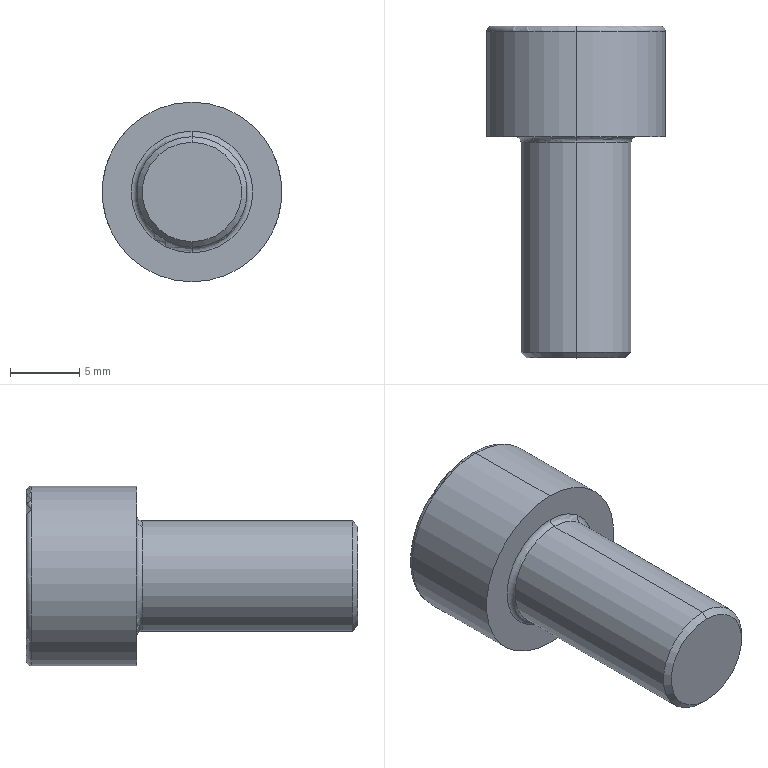Part | STEP file | 1 solid | 20 faces | box 13 x 24 x 13 mm | volume 1739 mm3 | plane 10 | torus 4 | cylinder 4 | cone 2 | commonest cylinder face diameters 8 x2 13 x2
STEP:
#1=CARTESIAN_POINT('',(0.,-16.,-3.6));
#2=VERTEX_POINT('',#1);
#3=CARTESIAN_POINT('',(0.,-16.,3.6));
#4=VERTEX_POINT('',#3);
#5=CARTESIAN_POINT('',(0.,-16.,0.));
#6=DIRECTION('',(0.,-1.,0.));
#7=DIRECTION('',(0.,0.,-1.));
#8=AXIS2_PLACEMENT_3D('',#5,#6,#7);
#9=CIRCLE('',#8,3.6);
#10=EDGE_CURVE('',#2,#4,#9,.T.);
#11=ORIENTED_EDGE('',*,*,#10,.F.);
#12=CARTESIAN_POINT('',(0.,-15.6,-4.));
#13=VERTEX_POINT('',#12);
#14=CARTESIAN_POINT('',(0.,-16.,-3.6));
#15=DIRECTION('',(0.,0.7071,-0.7071));
#16=VECTOR('',#15,1000.);
#17=LINE('',#14,#16);
#18=EDGE_CURVE('',#2,#13,#17,.T.);
#19=ORIENTED_EDGE('',*,*,#18,.T.);
#20=CARTESIAN_POINT('',(0.,-15.6,4.));
#21=VERTEX_POINT('',#20);
#22=CARTESIAN_POINT('',(0.,-15.6,0.));
#23=DIRECTION('',(0.,1.,0.));
#24=DIRECTION('',(0.,0.,-1.));
#25=AXIS2_PLACEMENT_3D('',#22,#23,#24);
#26=CIRCLE('',#25,4.);
#27=EDGE_CURVE('',#21,#13,#26,.T.);
#28=ORIENTED_EDGE('',*,*,#27,.F.);
#29=CARTESIAN_POINT('',(0.,-16.,3.6));
#30=DIRECTION('',(0.,0.7071,0.7071));
#31=VECTOR('',#30,1000.);
#32=LINE('',#29,#31);
#33=EDGE_CURVE('',#4,#21,#32,.T.);
#34=ORIENTED_EDGE('',*,*,#33,.F.);
#35=EDGE_LOOP('',(#11,#19,#28,#34));
#36=FACE_OUTER_BOUND('',#35,.T.);
#37=CARTESIAN_POINT('',(0.,-16.,0.));
#38=DIRECTION('',(0.,1.,0.));
#39=DIRECTION('',(0.,0.,1.));
#40=AXIS2_PLACEMENT_3D('',#37,#38,#39);
#41=CONICAL_SURFACE('',#40,3.6,0.7854);
#42=ADVANCED_FACE('',(#36),#41,.T.);
#43=CARTESIAN_POINT('',(0.,7.6,-6.5));
#44=VERTEX_POINT('',#43);
#45=CARTESIAN_POINT('',(0.,7.6,6.5));
#46=VERTEX_POINT('',#45);
#47=CARTESIAN_POINT('',(0.,7.6,0.));
#48=DIRECTION('',(0.,-1.,0.));
#49=DIRECTION('',(0.,0.,1.));
#50=AXIS2_PLACEMENT_3D('',#47,#48,#49);
#51=CIRCLE('',#50,6.5);
#52=EDGE_CURVE('',#44,#46,#51,.T.);
#53=ORIENTED_EDGE('',*,*,#52,.F.);
#54=CARTESIAN_POINT('',(0.,8.,-6.1));
#55=VERTEX_POINT('',#54);
#56=CARTESIAN_POINT('',(0.,7.6,-6.1));
#57=DIRECTION('',(1.,0.,0.));
#58=DIRECTION('',(0.,0.,-1.));
#59=AXIS2_PLACEMENT_3D('',#56,#57,#58);
#60=CIRCLE('',#59,0.4);
#61=EDGE_CURVE('',#44,#55,#60,.T.);
#62=ORIENTED_EDGE('',*,*,#61,.T.);
#63=CARTESIAN_POINT('',(0.,8.,6.1));
#64=VERTEX_POINT('',#63);
#65=CARTESIAN_POINT('',(0.,8.,0.));
#66=DIRECTION('',(0.,1.,0.));
#67=DIRECTION('',(0.,0.,1.));
#68=AXIS2_PLACEMENT_3D('',#65,#66,#67);
#69=CIRCLE('',#68,6.1);
#70=EDGE_CURVE('',#64,#55,#69,.T.);
#71=ORIENTED_EDGE('',*,*,#70,.F.);
#72=CARTESIAN_POINT('',(0.,7.6,6.1));
#73=DIRECTION('',(-1.,0.,0.));
#74=DIRECTION('',(0.,0.,1.));
#75=AXIS2_PLACEMENT_3D('',#72,#73,#74);
#76=CIRCLE('',#75,0.4);
#77=EDGE_CURVE('',#46,#64,#76,.T.);
#78=ORIENTED_EDGE('',*,*,#77,.F.);
#79=EDGE_LOOP('',(#53,#62,#71,#78));
#80=FACE_OUTER_BOUND('',#79,.T.);
#81=CARTESIAN_POINT('',(0.,7.6,0.));
#82=DIRECTION('',(0.,1.,0.));
#83=DIRECTION('',(0.,0.,1.));
#84=AXIS2_PLACEMENT_3D('',#81,#82,#83);
#85=TOROIDAL_SURFACE('',#84,6.1,0.4);
#86=ADVANCED_FACE('',(#80),#85,.T.);
#87=CARTESIAN_POINT('',(0.,-0.4,4.));
#88=VERTEX_POINT('',#87);
#89=CARTESIAN_POINT('',(0.,-0.4,-4.));
#90=VERTEX_POINT('',#89);
#91=CARTESIAN_POINT('',(0.,-0.4,0.));
#92=DIRECTION('',(0.,-1.,0.));
#93=DIRECTION('',(0.,0.,-1.));
#94=AXIS2_PLACEMENT_3D('',#91,#92,#93);
#95=CIRCLE('',#94,4.);
#96=EDGE_CURVE('',#88,#90,#95,.T.);
#97=ORIENTED_EDGE('',*,*,#96,.F.);
#98=CARTESIAN_POINT('',(0.,0.,4.4));
#99=VERTEX_POINT('',#98);
#100=CARTESIAN_POINT('',(0.,-0.4,4.4));
#101=DIRECTION('',(1.,0.,0.));
#102=DIRECTION('',(0.,0.,-1.));
#103=AXIS2_PLACEMENT_3D('',#100,#101,#102);
#104=CIRCLE('',#103,0.4);
#105=EDGE_CURVE('',#88,#99,#104,.T.);
#106=ORIENTED_EDGE('',*,*,#105,.T.);
#107=CARTESIAN_POINT('',(0.,0.,-4.4));
#108=VERTEX_POINT('',#107);
#109=CARTESIAN_POINT('',(0.,0.,0.));
#110=DIRECTION('',(0.,1.,0.));
#111=DIRECTION('',(0.,0.,-1.));
#112=AXIS2_PLACEMENT_3D('',#109,#110,#111);
#113=CIRCLE('',#112,4.4);
#114=EDGE_CURVE('',#108,#99,#113,.T.);
#115=ORIENTED_EDGE('',*,*,#114,.F.);
#116=CARTESIAN_POINT('',(0.,-0.4,-4.4));
#117=DIRECTION('',(-1.,0.,0.));
#118=DIRECTION('',(0.,0.,1.));
#119=AXIS2_PLACEMENT_3D('',#116,#117,#118);
#120=CIRCLE('',#119,0.4);
#121=EDGE_CURVE('',#90,#108,#120,.T.);
#122=ORIENTED_EDGE('',*,*,#121,.F.);
#123=EDGE_LOOP('',(#97,#106,#115,#122));
#124=FACE_OUTER_BOUND('',#123,.T.);
#125=CARTESIAN_POINT('',(0.,-0.4,0.));
#126=DIRECTION('',(0.,-1.,0.));
#127=DIRECTION('',(0.,0.,-1.));
#128=AXIS2_PLACEMENT_3D('',#125,#126,#127);
#129=TOROIDAL_SURFACE('',#128,4.4,0.4);
#130=ADVANCED_FACE('',(#124),#129,.F.);
#131=CARTESIAN_POINT('',(0.,-0.4,0.));
#132=DIRECTION('',(0.,-1.,0.));
#133=DIRECTION('',(0.,0.,-1.));
#134=AXIS2_PLACEMENT_3D('',#131,#132,#133);
#135=CIRCLE('',#134,4.);
#136=EDGE_CURVE('',#90,#88,#135,.T.);
#137=ORIENTED_EDGE('',*,*,#136,.T.);
#138=CARTESIAN_POINT('',(0.,0.,4.));
#139=DIRECTION('',(0.,-1.,0.));
#140=VECTOR('',#139,1000.);
#141=LINE('',#138,#140);
#142=EDGE_CURVE('',#88,#21,#141,.T.);
#143=ORIENTED_EDGE('',*,*,#142,.T.);
#144=ORIENTED_EDGE('',*,*,#27,.T.);
#145=CARTESIAN_POINT('',(0.,0.,-4.));
#146=DIRECTION('',(0.,-1.,0.));
#147=VECTOR('',#146,1000.);
#148=LINE('',#145,#147);
#149=EDGE_CURVE('',#90,#13,#148,.T.);
#150=ORIENTED_EDGE('',*,*,#149,.F.);
#151=EDGE_LOOP('',(#137,#143,#144,#150));
#152=FACE_OUTER_BOUND('',#151,.T.);
#153=CARTESIAN_POINT('',(0.,0.,0.));
#154=DIRECTION('',(0.,-1.,0.));
#155=DIRECTION('',(0.,0.,-1.));
#156=AXIS2_PLACEMENT_3D('',#153,#154,#155);
#157=CYLINDRICAL_SURFACE('',#156,4.);
#158=ADVANCED_FACE('',(#152),#157,.T.);
#159=ORIENTED_EDGE('',*,*,#52,.T.);
#160=CARTESIAN_POINT('',(0.,0.,6.5));
#161=VERTEX_POINT('',#160);
#162=CARTESIAN_POINT('',(0.,0.,6.5));
#163=DIRECTION('',(0.,-1.,0.));
#164=VECTOR('',#163,1000.);
#165=LINE('',#162,#164);
#166=EDGE_CURVE('',#46,#161,#165,.T.);
#167=ORIENTED_EDGE('',*,*,#166,.T.);
#168=CARTESIAN_POINT('',(0.,0.,-6.5));
#169=VERTEX_POINT('',#168);
#170=CARTESIAN_POINT('',(0.,0.,0.));
#171=DIRECTION('',(0.,-1.,0.));
#172=DIRECTION('',(0.,0.,-1.));
#173=AXIS2_PLACEMENT_3D('',#170,#171,#172);
#174=CIRCLE('',#173,6.5);
#175=EDGE_CURVE('',#169,#161,#174,.T.);
#176=ORIENTED_EDGE('',*,*,#175,.F.);
#177=CARTESIAN_POINT('',(0.,0.,-6.5));
#178=DIRECTION('',(0.,-1.,0.));
#179=VECTOR('',#178,1000.);
#180=LINE('',#177,#179);
#181=EDGE_CURVE('',#44,#169,#180,.T.);
#182=ORIENTED_EDGE('',*,*,#181,.F.);
#183=EDGE_LOOP('',(#159,#167,#176,#182));
#184=FACE_OUTER_BOUND('',#183,.T.);
#185=CARTESIAN_POINT('',(0.,0.,0.));
#186=DIRECTION('',(0.,-1.,0.));
#187=DIRECTION('',(0.,0.,-1.));
#188=AXIS2_PLACEMENT_3D('',#185,#186,#187);
#189=CYLINDRICAL_SURFACE('',#188,6.5);
#190=ADVANCED_FACE('',(#184),#189,.T.);
#191=ORIENTED_EDGE('',*,*,#70,.T.);
#192=CARTESIAN_POINT('',(0.,8.,0.));
#193=DIRECTION('',(0.,1.,0.));
#194=DIRECTION('',(0.,0.,1.));
#195=AXIS2_PLACEMENT_3D('',#192,#193,#194);
#196=CIRCLE('',#195,6.1);
#197=EDGE_CURVE('',#55,#64,#196,.T.);
#198=ORIENTED_EDGE('',*,*,#197,.T.);
#199=EDGE_LOOP('',(#191,#198));
#200=FACE_OUTER_BOUND('',#199,.T.);
#201=CARTESIAN_POINT('',(0.,8.,-3.464));
#202=VERTEX_POINT('',#201);
#203=CARTESIAN_POINT('',(-3.,8.,-1.732));
#204=VERTEX_POINT('',#203);
#205=CARTESIAN_POINT('',(0.,8.,-3.464));
#206=DIRECTION('',(-0.866,0.,0.5));
#207=VECTOR('',#206,1000.);
#208=LINE('',#205,#207);
#209=EDGE_CURVE('',#202,#204,#208,.T.);
#210=ORIENTED_EDGE('',*,*,#209,.F.);
#211=CARTESIAN_POINT('',(3.,8.,-1.732));
#212=VERTEX_POINT('',#211);
#213=CARTESIAN_POINT('',(3.,8.,-1.732));
#214=DIRECTION('',(-0.866,0.,-0.5));
#215=VECTOR('',#214,1000.);
#216=LINE('',#213,#215);
#217=EDGE_CURVE('',#212,#202,#216,.T.);
#218=ORIENTED_EDGE('',*,*,#217,.F.);
#219=CARTESIAN_POINT('',(3.,8.,1.732));
#220=VERTEX_POINT('',#219);
#221=CARTESIAN_POINT('',(3.,8.,1.732));
#222=DIRECTION('',(0.,0.,-1.));
#223=VECTOR('',#222,1000.);
#224=LINE('',#221,#223);
#225=EDGE_CURVE('',#220,#212,#224,.T.);
#226=ORIENTED_EDGE('',*,*,#225,.F.);
#227=CARTESIAN_POINT('',(0.,8.,3.464));
#228=VERTEX_POINT('',#227);
#229=CARTESIAN_POINT('',(0.,8.,3.464));
#230=DIRECTION('',(0.866,0.,-0.5));
#231=VECTOR('',#230,1000.);
#232=LINE('',#229,#231);
#233=EDGE_CURVE('',#228,#220,#232,.T.);
#234=ORIENTED_EDGE('',*,*,#233,.F.);
#235=CARTESIAN_POINT('',(-3.,8.,1.732));
#236=VERTEX_POINT('',#235);
#237=CARTESIAN_POINT('',(-3.,8.,1.732));
#238=DIRECTION('',(0.866,0.,0.5));
#239=VECTOR('',#238,1000.);
#240=LINE('',#237,#239);
#241=EDGE_CURVE('',#236,#228,#240,.T.);
#242=ORIENTED_EDGE('',*,*,#241,.F.);
#243=CARTESIAN_POINT('',(-3.,8.,-1.732));
#244=DIRECTION('',(0.,0.,1.));
#245=VECTOR('',#244,1000.);
#246=LINE('',#243,#245);
#247=EDGE_CURVE('',#204,#236,#246,.T.);
#248=ORIENTED_EDGE('',*,*,#247,.F.);
#249=EDGE_LOOP('',(#210,#218,#226,#234,#242,#248));
#250=FACE_BOUND('',#249,.T.);
#251=CARTESIAN_POINT('',(0.,8.,0.));
#252=DIRECTION('',(0.,1.,0.));
#253=DIRECTION('',(0.,0.,1.));
#254=AXIS2_PLACEMENT_3D('',#251,#252,#253);
#255=PLANE('',#254);
#256=ADVANCED_FACE('',(#200,#250),#255,.T.);
#257=ORIENTED_EDGE('',*,*,#166,.F.);
#258=CARTESIAN_POINT('',(0.,7.6,0.));
#259=DIRECTION('',(0.,-1.,0.));
#260=DIRECTION('',(0.,0.,1.));
#261=AXIS2_PLACEMENT_3D('',#258,#259,#260);
#262=CIRCLE('',#261,6.5);
#263=EDGE_CURVE('',#46,#44,#262,.T.);
#264=ORIENTED_EDGE('',*,*,#263,.T.);
#265=ORIENTED_EDGE('',*,*,#181,.T.);
#266=CARTESIAN_POINT('',(0.,0.,0.));
#267=DIRECTION('',(0.,-1.,0.));
#268=DIRECTION('',(0.,0.,-1.));
#269=AXIS2_PLACEMENT_3D('',#266,#267,#268);
#270=CIRCLE('',#269,6.5);
#271=EDGE_CURVE('',#161,#169,#270,.T.);
#272=ORIENTED_EDGE('',*,*,#271,.F.);
#273=EDGE_LOOP('',(#257,#264,#265,#272));
#274=FACE_OUTER_BOUND('',#273,.T.);
#275=CARTESIAN_POINT('',(0.,0.,0.));
#276=DIRECTION('',(0.,-1.,0.));
#277=DIRECTION('',(0.,0.,-1.));
#278=AXIS2_PLACEMENT_3D('',#275,#276,#277);
#279=CYLINDRICAL_SURFACE('',#278,6.5);
#280=ADVANCED_FACE('',(#274),#279,.T.);
#281=ORIENTED_EDGE('',*,*,#114,.T.);
#282=CARTESIAN_POINT('',(0.,0.,0.));
#283=DIRECTION('',(0.,1.,0.));
#284=DIRECTION('',(0.,0.,-1.));
#285=AXIS2_PLACEMENT_3D('',#282,#283,#284);
#286=CIRCLE('',#285,4.4);
#287=EDGE_CURVE('',#99,#108,#286,.T.);
#288=ORIENTED_EDGE('',*,*,#287,.T.);
#289=EDGE_LOOP('',(#281,#288));
#290=FACE_BOUND('',#289,.T.);
#291=ORIENTED_EDGE('',*,*,#175,.T.);
#292=ORIENTED_EDGE('',*,*,#271,.T.);
#293=EDGE_LOOP('',(#291,#292));
#294=FACE_OUTER_BOUND('',#293,.T.);
#295=CARTESIAN_POINT('',(6.5,0.,0.));
#296=DIRECTION('',(0.,-1.,0.));
#297=DIRECTION('',(0.,0.,-1.));
#298=AXIS2_PLACEMENT_3D('',#295,#296,#297);
#299=PLANE('',#298);
#300=ADVANCED_FACE('',(#290,#294),#299,.T.);
#301=ORIENTED_EDGE('',*,*,#142,.F.);
#302=ORIENTED_EDGE('',*,*,#96,.T.);
#303=ORIENTED_EDGE('',*,*,#149,.T.);
#304=CARTESIAN_POINT('',(0.,-15.6,0.));
#305=DIRECTION('',(0.,1.,0.));
#306=DIRECTION('',(0.,0.,-1.));
#307=AXIS2_PLACEMENT_3D('',#304,#305,#306);
#308=CIRCLE('',#307,4.);
#309=EDGE_CURVE('',#13,#21,#308,.T.);
#310=ORIENTED_EDGE('',*,*,#309,.T.);
#311=EDGE_LOOP('',(#301,#302,#303,#310));
#312=FACE_OUTER_BOUND('',#311,.T.);
#313=CARTESIAN_POINT('',(0.,0.,0.));
#314=DIRECTION('',(0.,-1.,0.));
#315=DIRECTION('',(0.,0.,-1.));
#316=AXIS2_PLACEMENT_3D('',#313,#314,#315);
#317=CYLINDRICAL_SURFACE('',#316,4.);
#318=ADVANCED_FACE('',(#312),#317,.T.);
#319=CARTESIAN_POINT('',(0.,-16.,0.));
#320=DIRECTION('',(0.,-1.,0.));
#321=DIRECTION('',(0.,0.,-1.));
#322=AXIS2_PLACEMENT_3D('',#319,#320,#321);
#323=CIRCLE('',#322,3.6);
#324=EDGE_CURVE('',#4,#2,#323,.T.);
#325=ORIENTED_EDGE('',*,*,#324,.T.);
#326=ORIENTED_EDGE('',*,*,#10,.T.);
#327=EDGE_LOOP('',(#325,#326));
#328=FACE_OUTER_BOUND('',#327,.T.);
#329=CARTESIAN_POINT('',(4.,-16.,0.));
#330=DIRECTION('',(0.,-1.,0.));
#331=DIRECTION('',(0.,0.,-1.));
#332=AXIS2_PLACEMENT_3D('',#329,#330,#331);
#333=PLANE('',#332);
#334=ADVANCED_FACE('',(#328),#333,.T.);
#335=ORIENTED_EDGE('',*,*,#209,.T.);
#336=CARTESIAN_POINT('',(-3.,4.,-1.732));
#337=VERTEX_POINT('',#336);
#338=CARTESIAN_POINT('',(-3.,4.,-1.732));
#339=DIRECTION('',(0.,1.,0.));
#340=VECTOR('',#339,1000.);
#341=LINE('',#338,#340);
#342=EDGE_CURVE('',#337,#204,#341,.T.);
#343=ORIENTED_EDGE('',*,*,#342,.F.);
#344=CARTESIAN_POINT('',(0.,4.,-3.464));
#345=VERTEX_POINT('',#344);
#346=CARTESIAN_POINT('',(0.,4.,-3.464));
#347=DIRECTION('',(-0.866,0.,0.5));
#348=VECTOR('',#347,1000.);
#349=LINE('',#346,#348);
#350=EDGE_CURVE('',#345,#337,#349,.T.);
#351=ORIENTED_EDGE('',*,*,#350,.F.);
#352=CARTESIAN_POINT('',(0.,4.,-3.464));
#353=DIRECTION('',(0.,1.,0.));
#354=VECTOR('',#353,1000.);
#355=LINE('',#352,#354);
#356=EDGE_CURVE('',#345,#202,#355,.T.);
#357=ORIENTED_EDGE('',*,*,#356,.T.);
#358=EDGE_LOOP('',(#335,#343,#351,#357));
#359=FACE_OUTER_BOUND('',#358,.T.);
#360=CARTESIAN_POINT('',(0.,4.,-3.464));
#361=DIRECTION('',(-0.5,0.,-0.866));
#362=DIRECTION('',(-0.866,0.,0.5));
#363=AXIS2_PLACEMENT_3D('',#360,#361,#362);
#364=PLANE('',#363);
#365=ADVANCED_FACE('',(#359),#364,.F.);
#366=ORIENTED_EDGE('',*,*,#217,.T.);
#367=ORIENTED_EDGE('',*,*,#356,.F.);
#368=CARTESIAN_POINT('',(3.,4.,-1.732));
#369=VERTEX_POINT('',#368);
#370=CARTESIAN_POINT('',(3.,4.,-1.732));
#371=DIRECTION('',(-0.866,0.,-0.5));
#372=VECTOR('',#371,1000.);
#373=LINE('',#370,#372);
#374=EDGE_CURVE('',#369,#345,#373,.T.);
#375=ORIENTED_EDGE('',*,*,#374,.F.);
#376=CARTESIAN_POINT('',(3.,4.,-1.732));
#377=DIRECTION('',(0.,1.,0.));
#378=VECTOR('',#377,1000.);
#379=LINE('',#376,#378);
#380=EDGE_CURVE('',#369,#212,#379,.T.);
#381=ORIENTED_EDGE('',*,*,#380,.T.);
#382=EDGE_LOOP('',(#366,#367,#375,#381));
#383=FACE_OUTER_BOUND('',#382,.T.);
#384=CARTESIAN_POINT('',(3.,4.,-1.732));
#385=DIRECTION('',(0.5,0.,-0.866));
#386=DIRECTION('',(-0.866,0.,-0.5));
#387=AXIS2_PLACEMENT_3D('',#384,#385,#386);
#388=PLANE('',#387);
#389=ADVANCED_FACE('',(#383),#388,.F.);
#390=ORIENTED_EDGE('',*,*,#225,.T.);
#391=ORIENTED_EDGE('',*,*,#380,.F.);
#392=CARTESIAN_POINT('',(3.,4.,1.732));
#393=VERTEX_POINT('',#392);
#394=CARTESIAN_POINT('',(3.,4.,1.732));
#395=DIRECTION('',(0.,0.,-1.));
#396=VECTOR('',#395,1000.);
#397=LINE('',#394,#396);
#398=EDGE_CURVE('',#393,#369,#397,.T.);
#399=ORIENTED_EDGE('',*,*,#398,.F.);
#400=CARTESIAN_POINT('',(3.,4.,1.732));
#401=DIRECTION('',(0.,1.,0.));
#402=VECTOR('',#401,1000.);
#403=LINE('',#400,#402);
#404=EDGE_CURVE('',#393,#220,#403,.T.);
#405=ORIENTED_EDGE('',*,*,#404,.T.);
#406=EDGE_LOOP('',(#390,#391,#399,#405));
#407=FACE_OUTER_BOUND('',#406,.T.);
#408=CARTESIAN_POINT('',(3.,4.,1.732));
#409=DIRECTION('',(1.,0.,0.));
#410=DIRECTION('',(0.,0.,-1.));
#411=AXIS2_PLACEMENT_3D('',#408,#409,#410);
#412=PLANE('',#411);
#413=ADVANCED_FACE('',(#407),#412,.F.);
#414=ORIENTED_EDGE('',*,*,#233,.T.);
#415=ORIENTED_EDGE('',*,*,#404,.F.);
#416=CARTESIAN_POINT('',(0.,4.,3.464));
#417=VERTEX_POINT('',#416);
#418=CARTESIAN_POINT('',(0.,4.,3.464));
#419=DIRECTION('',(0.866,0.,-0.5));
#420=VECTOR('',#419,1000.);
#421=LINE('',#418,#420);
#422=EDGE_CURVE('',#417,#393,#421,.T.);
#423=ORIENTED_EDGE('',*,*,#422,.F.);
#424=CARTESIAN_POINT('',(0.,4.,3.464));
#425=DIRECTION('',(0.,1.,0.));
#426=VECTOR('',#425,1000.);
#427=LINE('',#424,#426);
#428=EDGE_CURVE('',#417,#228,#427,.T.);
#429=ORIENTED_EDGE('',*,*,#428,.T.);
#430=EDGE_LOOP('',(#414,#415,#423,#429));
#431=FACE_OUTER_BOUND('',#430,.T.);
#432=CARTESIAN_POINT('',(0.,4.,3.464));
#433=DIRECTION('',(0.5,0.,0.866));
#434=DIRECTION('',(0.866,0.,-0.5));
#435=AXIS2_PLACEMENT_3D('',#432,#433,#434);
#436=PLANE('',#435);
#437=ADVANCED_FACE('',(#431),#436,.F.);
#438=ORIENTED_EDGE('',*,*,#241,.T.);
#439=ORIENTED_EDGE('',*,*,#428,.F.);
#440=CARTESIAN_POINT('',(-3.,4.,1.732));
#441=VERTEX_POINT('',#440);
#442=CARTESIAN_POINT('',(-3.,4.,1.732));
#443=DIRECTION('',(0.866,0.,0.5));
#444=VECTOR('',#443,1000.);
#445=LINE('',#442,#444);
#446=EDGE_CURVE('',#441,#417,#445,.T.);
#447=ORIENTED_EDGE('',*,*,#446,.F.);
#448=CARTESIAN_POINT('',(-3.,4.,1.732));
#449=DIRECTION('',(0.,1.,0.));
#450=VECTOR('',#449,1000.);
#451=LINE('',#448,#450);
#452=EDGE_CURVE('',#441,#236,#451,.T.);
#453=ORIENTED_EDGE('',*,*,#452,.T.);
#454=EDGE_LOOP('',(#438,#439,#447,#453));
#455=FACE_OUTER_BOUND('',#454,.T.);
#456=CARTESIAN_POINT('',(-3.,4.,1.732));
#457=DIRECTION('',(-0.5,0.,0.866));
#458=DIRECTION('',(0.866,0.,0.5));
#459=AXIS2_PLACEMENT_3D('',#456,#457,#458);
#460=PLANE('',#459);
#461=ADVANCED_FACE('',(#455),#460,.F.);
#462=ORIENTED_EDGE('',*,*,#247,.T.);
#463=ORIENTED_EDGE('',*,*,#452,.F.);
#464=CARTESIAN_POINT('',(-3.,4.,-1.732));
#465=DIRECTION('',(0.,0.,1.));
#466=VECTOR('',#465,1000.);
#467=LINE('',#464,#466);
#468=EDGE_CURVE('',#337,#441,#467,.T.);
#469=ORIENTED_EDGE('',*,*,#468,.F.);
#470=ORIENTED_EDGE('',*,*,#342,.T.);
#471=EDGE_LOOP('',(#462,#463,#469,#470));
#472=FACE_OUTER_BOUND('',#471,.T.);
#473=CARTESIAN_POINT('',(-3.,4.,-1.732));
#474=DIRECTION('',(-1.,0.,0.));
#475=DIRECTION('',(0.,0.,1.));
#476=AXIS2_PLACEMENT_3D('',#473,#474,#475);
#477=PLANE('',#476);
#478=ADVANCED_FACE('',(#472),#477,.F.);
#479=ORIENTED_EDGE('',*,*,#350,.T.);
#480=ORIENTED_EDGE('',*,*,#468,.T.);
#481=ORIENTED_EDGE('',*,*,#446,.T.);
#482=ORIENTED_EDGE('',*,*,#422,.T.);
#483=ORIENTED_EDGE('',*,*,#398,.T.);
#484=ORIENTED_EDGE('',*,*,#374,.T.);
#485=EDGE_LOOP('',(#479,#480,#481,#482,#483,#484));
#486=FACE_OUTER_BOUND('',#485,.T.);
#487=CARTESIAN_POINT('',(0.,4.,0.));
#488=DIRECTION('',(0.,1.,0.));
#489=DIRECTION('',(0.,0.,1.));
#490=AXIS2_PLACEMENT_3D('',#487,#488,#489);
#491=PLANE('',#490);
#492=ADVANCED_FACE('',(#486),#491,.T.);
#493=ORIENTED_EDGE('',*,*,#105,.F.);
#494=ORIENTED_EDGE('',*,*,#136,.F.);
#495=ORIENTED_EDGE('',*,*,#121,.T.);
#496=ORIENTED_EDGE('',*,*,#287,.F.);
#497=EDGE_LOOP('',(#493,#494,#495,#496));
#498=FACE_OUTER_BOUND('',#497,.T.);
#499=CARTESIAN_POINT('',(0.,-0.4,0.));
#500=DIRECTION('',(0.,-1.,0.));
#501=DIRECTION('',(0.,0.,-1.));
#502=AXIS2_PLACEMENT_3D('',#499,#500,#501);
#503=TOROIDAL_SURFACE('',#502,4.4,0.4);
#504=ADVANCED_FACE('',(#498),#503,.F.);
#505=ORIENTED_EDGE('',*,*,#61,.F.);
#506=ORIENTED_EDGE('',*,*,#263,.F.);
#507=ORIENTED_EDGE('',*,*,#77,.T.);
#508=ORIENTED_EDGE('',*,*,#197,.F.);
#509=EDGE_LOOP('',(#505,#506,#507,#508));
#510=FACE_OUTER_BOUND('',#509,.T.);
#511=CARTESIAN_POINT('',(0.,7.6,0.));
#512=DIRECTION('',(0.,1.,0.));
#513=DIRECTION('',(0.,0.,1.));
#514=AXIS2_PLACEMENT_3D('',#511,#512,#513);
#515=TOROIDAL_SURFACE('',#514,6.1,0.4);
#516=ADVANCED_FACE('',(#510),#515,.T.);
#517=ORIENTED_EDGE('',*,*,#18,.F.);
#518=ORIENTED_EDGE('',*,*,#324,.F.);
#519=ORIENTED_EDGE('',*,*,#33,.T.);
#520=ORIENTED_EDGE('',*,*,#309,.F.);
#521=EDGE_LOOP('',(#517,#518,#519,#520));
#522=FACE_OUTER_BOUND('',#521,.T.);
#523=CARTESIAN_POINT('',(0.,-16.,0.));
#524=DIRECTION('',(0.,1.,0.));
#525=DIRECTION('',(0.,0.,1.));
#526=AXIS2_PLACEMENT_3D('',#523,#524,#525);
#527=CONICAL_SURFACE('',#526,3.6,0.7854);
#528=ADVANCED_FACE('',(#522),#527,.T.);
#529=CLOSED_SHELL('',(#42,#86,#130,#158,#190,#256,#280,#300,#318,#334,#365,#389,#413,#437,#461,#478,#492,#504,#516,#528));
#530=MANIFOLD_SOLID_BREP('',#529);
#531=CARTESIAN_POINT('',(0.,0.,0.));
#532=DIRECTION('',(0.,0.,1.));
#533=DIRECTION('',(1.,0.,0.));
#534=AXIS2_PLACEMENT_3D('',#531,#532,#533);
#535=(LENGTH_UNIT()NAMED_UNIT(*)SI_UNIT(.MILLI.,.METRE.));
#536=UNCERTAINTY_MEASURE_WITH_UNIT(LENGTH_MEASURE(0.00001),#535,'','');
#537=(NAMED_UNIT(*)PLANE_ANGLE_UNIT()SI_UNIT($,.RADIAN.));
#538=(NAMED_UNIT(*)SI_UNIT($,.STERADIAN.)SOLID_ANGLE_UNIT());
#539=(GEOMETRIC_REPRESENTATION_CONTEXT(3)GLOBAL_UNCERTAINTY_ASSIGNED_CONTEXT((#536))GLOBAL_UNIT_ASSIGNED_CONTEXT((#535,#537,#538))REPRESENTATION_CONTEXT('',''));
#540=ADVANCED_BREP_SHAPE_REPRESENTATION('',(#530,#534),#539);